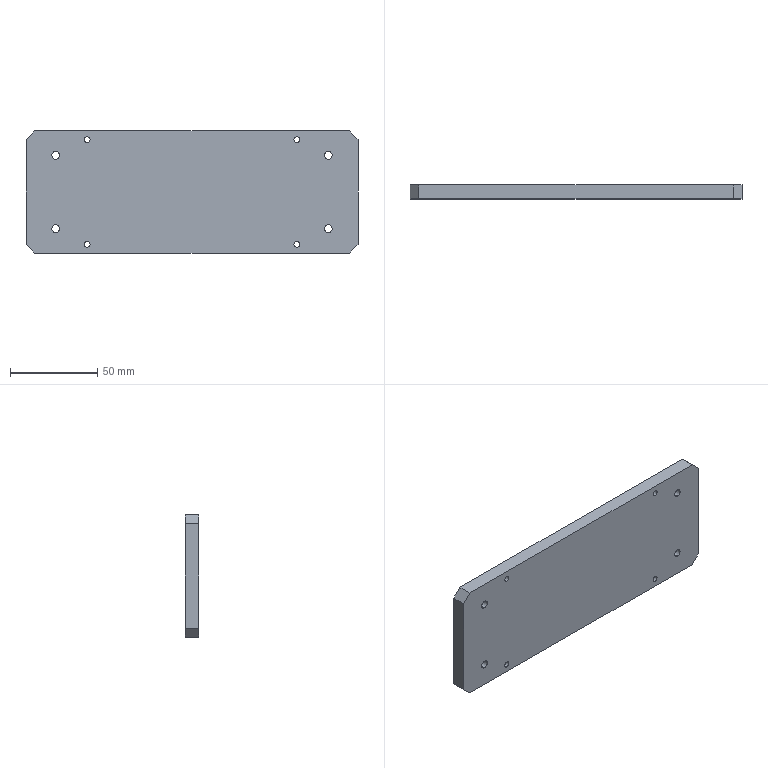Part | STEP file | PN_0030 | 1 solid | 38 faces | box 190 x 8 x 70 mm | volume 104613 mm3 | cylinder 24 | plane 14 | commonest cylinder face diameters 3.3 x8 4.5 x8 8 x8